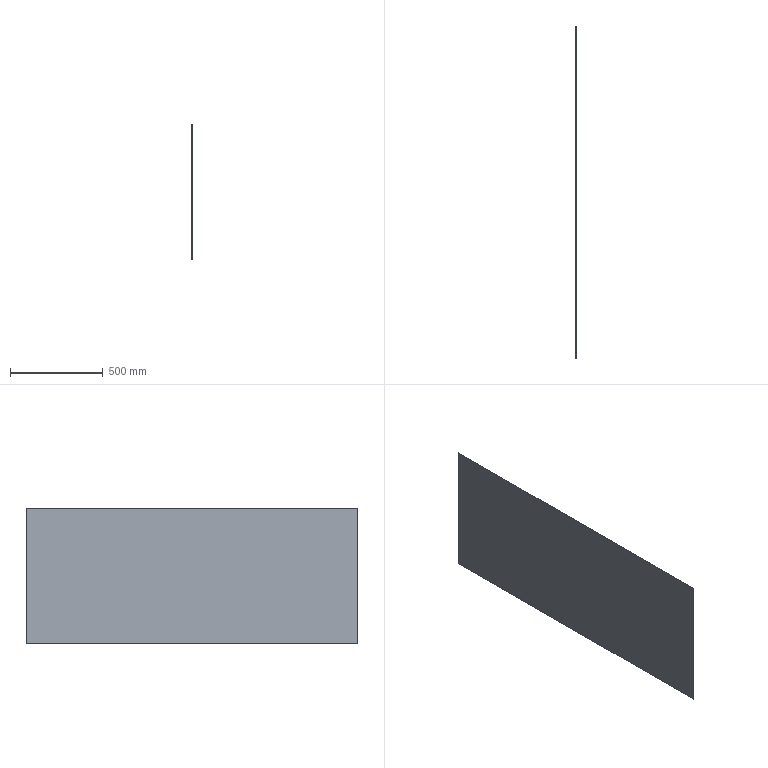Part | SolidWorks | 1 solid | 6 faces | box 1.5 x 1790 x 730 mm | volume 1960050 mm3 | plane 6
STEP:
#1=CARTESIAN_POINT('',(0.,895.,365.));
#2=VERTEX_POINT('',#1);
#3=CARTESIAN_POINT('',(0.,-895.,365.));
#4=VERTEX_POINT('',#3);
#5=CARTESIAN_POINT('',(0.,-895.,365.));
#6=DIRECTION('',(0.,-1.,0.));
#7=VECTOR('',#6,1000.);
#8=LINE('',#5,#7);
#9=EDGE_CURVE('',#2,#4,#8,.T.);
#10=ORIENTED_EDGE('',*,*,#9,.F.);
#11=CARTESIAN_POINT('',(-1.5,895.,365.));
#12=VERTEX_POINT('',#11);
#13=CARTESIAN_POINT('',(-1.5,895.,365.));
#14=DIRECTION('',(1.,0.,0.));
#15=VECTOR('',#14,1000.);
#16=LINE('',#13,#15);
#17=EDGE_CURVE('',#12,#2,#16,.T.);
#18=ORIENTED_EDGE('',*,*,#17,.F.);
#19=CARTESIAN_POINT('',(-1.5,-895.,365.));
#20=VERTEX_POINT('',#19);
#21=CARTESIAN_POINT('',(-1.5,-895.,365.));
#22=DIRECTION('',(0.,-1.,0.));
#23=VECTOR('',#22,1000.);
#24=LINE('',#21,#23);
#25=EDGE_CURVE('',#12,#20,#24,.T.);
#26=ORIENTED_EDGE('',*,*,#25,.T.);
#27=CARTESIAN_POINT('',(-1.5,-895.,365.));
#28=DIRECTION('',(1.,0.,0.));
#29=VECTOR('',#28,1000.);
#30=LINE('',#27,#29);
#31=EDGE_CURVE('',#20,#4,#30,.T.);
#32=ORIENTED_EDGE('',*,*,#31,.T.);
#33=EDGE_LOOP('',(#10,#18,#26,#32));
#34=FACE_OUTER_BOUND('',#33,.T.);
#35=CARTESIAN_POINT('',(-1.5,-895.,365.));
#36=DIRECTION('',(0.,0.,1.));
#37=DIRECTION('',(1.,0.,0.));
#38=AXIS2_PLACEMENT_3D('',#35,#36,#37);
#39=PLANE('',#38);
#40=ADVANCED_FACE('',(#34),#39,.T.);
#41=CARTESIAN_POINT('',(0.,895.,-365.));
#42=VERTEX_POINT('',#41);
#43=CARTESIAN_POINT('',(0.,895.,-365.));
#44=DIRECTION('',(0.,0.,1.));
#45=VECTOR('',#44,1000.);
#46=LINE('',#43,#45);
#47=EDGE_CURVE('',#42,#2,#46,.T.);
#48=ORIENTED_EDGE('',*,*,#47,.F.);
#49=CARTESIAN_POINT('',(-1.5,895.,-365.));
#50=VERTEX_POINT('',#49);
#51=CARTESIAN_POINT('',(-1.5,895.,-365.));
#52=DIRECTION('',(1.,0.,0.));
#53=VECTOR('',#52,1000.);
#54=LINE('',#51,#53);
#55=EDGE_CURVE('',#50,#42,#54,.T.);
#56=ORIENTED_EDGE('',*,*,#55,.F.);
#57=CARTESIAN_POINT('',(-1.5,895.,-365.));
#58=DIRECTION('',(0.,0.,1.));
#59=VECTOR('',#58,1000.);
#60=LINE('',#57,#59);
#61=EDGE_CURVE('',#50,#12,#60,.T.);
#62=ORIENTED_EDGE('',*,*,#61,.T.);
#63=ORIENTED_EDGE('',*,*,#17,.T.);
#64=EDGE_LOOP('',(#48,#56,#62,#63));
#65=FACE_OUTER_BOUND('',#64,.T.);
#66=CARTESIAN_POINT('',(-1.5,895.,-365.));
#67=DIRECTION('',(0.,1.,0.));
#68=DIRECTION('',(0.,0.,1.));
#69=AXIS2_PLACEMENT_3D('',#66,#67,#68);
#70=PLANE('',#69);
#71=ADVANCED_FACE('',(#65),#70,.T.);
#72=CARTESIAN_POINT('',(0.,-895.,-365.));
#73=VERTEX_POINT('',#72);
#74=CARTESIAN_POINT('',(0.,-895.,-365.));
#75=DIRECTION('',(0.,1.,0.));
#76=VECTOR('',#75,1000.);
#77=LINE('',#74,#76);
#78=EDGE_CURVE('',#73,#42,#77,.T.);
#79=ORIENTED_EDGE('',*,*,#78,.F.);
#80=CARTESIAN_POINT('',(-1.5,-895.,-365.));
#81=VERTEX_POINT('',#80);
#82=CARTESIAN_POINT('',(-1.5,-895.,-365.));
#83=DIRECTION('',(1.,0.,0.));
#84=VECTOR('',#83,1000.);
#85=LINE('',#82,#84);
#86=EDGE_CURVE('',#81,#73,#85,.T.);
#87=ORIENTED_EDGE('',*,*,#86,.F.);
#88=CARTESIAN_POINT('',(-1.5,-895.,-365.));
#89=DIRECTION('',(0.,1.,0.));
#90=VECTOR('',#89,1000.);
#91=LINE('',#88,#90);
#92=EDGE_CURVE('',#81,#50,#91,.T.);
#93=ORIENTED_EDGE('',*,*,#92,.T.);
#94=ORIENTED_EDGE('',*,*,#55,.T.);
#95=EDGE_LOOP('',(#79,#87,#93,#94));
#96=FACE_OUTER_BOUND('',#95,.T.);
#97=CARTESIAN_POINT('',(-1.5,-895.,-365.));
#98=DIRECTION('',(0.,0.,-1.));
#99=DIRECTION('',(-1.,0.,0.));
#100=AXIS2_PLACEMENT_3D('',#97,#98,#99);
#101=PLANE('',#100);
#102=ADVANCED_FACE('',(#96),#101,.T.);
#103=CARTESIAN_POINT('',(0.,-895.,-365.));
#104=DIRECTION('',(0.,0.,-1.));
#105=VECTOR('',#104,1000.);
#106=LINE('',#103,#105);
#107=EDGE_CURVE('',#4,#73,#106,.T.);
#108=ORIENTED_EDGE('',*,*,#107,.F.);
#109=ORIENTED_EDGE('',*,*,#31,.F.);
#110=CARTESIAN_POINT('',(-1.5,-895.,-365.));
#111=DIRECTION('',(0.,0.,-1.));
#112=VECTOR('',#111,1000.);
#113=LINE('',#110,#112);
#114=EDGE_CURVE('',#20,#81,#113,.T.);
#115=ORIENTED_EDGE('',*,*,#114,.T.);
#116=ORIENTED_EDGE('',*,*,#86,.T.);
#117=EDGE_LOOP('',(#108,#109,#115,#116));
#118=FACE_OUTER_BOUND('',#117,.T.);
#119=CARTESIAN_POINT('',(-1.5,-895.,-365.));
#120=DIRECTION('',(0.,-1.,0.));
#121=DIRECTION('',(0.,0.,-1.));
#122=AXIS2_PLACEMENT_3D('',#119,#120,#121);
#123=PLANE('',#122);
#124=ADVANCED_FACE('',(#118),#123,.T.);
#125=ORIENTED_EDGE('',*,*,#25,.F.);
#126=ORIENTED_EDGE('',*,*,#61,.F.);
#127=ORIENTED_EDGE('',*,*,#92,.F.);
#128=ORIENTED_EDGE('',*,*,#114,.F.);
#129=EDGE_LOOP('',(#125,#126,#127,#128));
#130=FACE_OUTER_BOUND('',#129,.T.);
#131=CARTESIAN_POINT('',(-1.5,0.,0.));
#132=DIRECTION('',(1.,0.,0.));
#133=DIRECTION('',(0.,0.,-1.));
#134=AXIS2_PLACEMENT_3D('',#131,#132,#133);
#135=PLANE('',#134);
#136=ADVANCED_FACE('',(#130),#135,.F.);
#137=ORIENTED_EDGE('',*,*,#9,.T.);
#138=ORIENTED_EDGE('',*,*,#107,.T.);
#139=ORIENTED_EDGE('',*,*,#78,.T.);
#140=ORIENTED_EDGE('',*,*,#47,.T.);
#141=EDGE_LOOP('',(#137,#138,#139,#140));
#142=FACE_OUTER_BOUND('',#141,.T.);
#143=CARTESIAN_POINT('',(0.,0.,0.));
#144=DIRECTION('',(1.,0.,0.));
#145=DIRECTION('',(0.,0.,-1.));
#146=AXIS2_PLACEMENT_3D('',#143,#144,#145);
#147=PLANE('',#146);
#148=ADVANCED_FACE('',(#142),#147,.T.);
#149=CLOSED_SHELL('',(#40,#71,#102,#124,#136,#148));
#150=MANIFOLD_SOLID_BREP('',#149);
#151=CARTESIAN_POINT('',(0.,0.,0.));
#152=DIRECTION('',(0.,0.,1.));
#153=DIRECTION('',(1.,0.,0.));
#154=AXIS2_PLACEMENT_3D('',#151,#152,#153);
#155=(LENGTH_UNIT()NAMED_UNIT(*)SI_UNIT(.MILLI.,.METRE.));
#156=UNCERTAINTY_MEASURE_WITH_UNIT(LENGTH_MEASURE(0.00001),#155,'','');
#157=(NAMED_UNIT(*)PLANE_ANGLE_UNIT()SI_UNIT($,.RADIAN.));
#158=(NAMED_UNIT(*)SI_UNIT($,.STERADIAN.)SOLID_ANGLE_UNIT());
#159=(GEOMETRIC_REPRESENTATION_CONTEXT(3)GLOBAL_UNCERTAINTY_ASSIGNED_CONTEXT((#156))GLOBAL_UNIT_ASSIGNED_CONTEXT((#155,#157,#158))REPRESENTATION_CONTEXT('',''));
#160=ADVANCED_BREP_SHAPE_REPRESENTATION('',(#150,#154),#159);